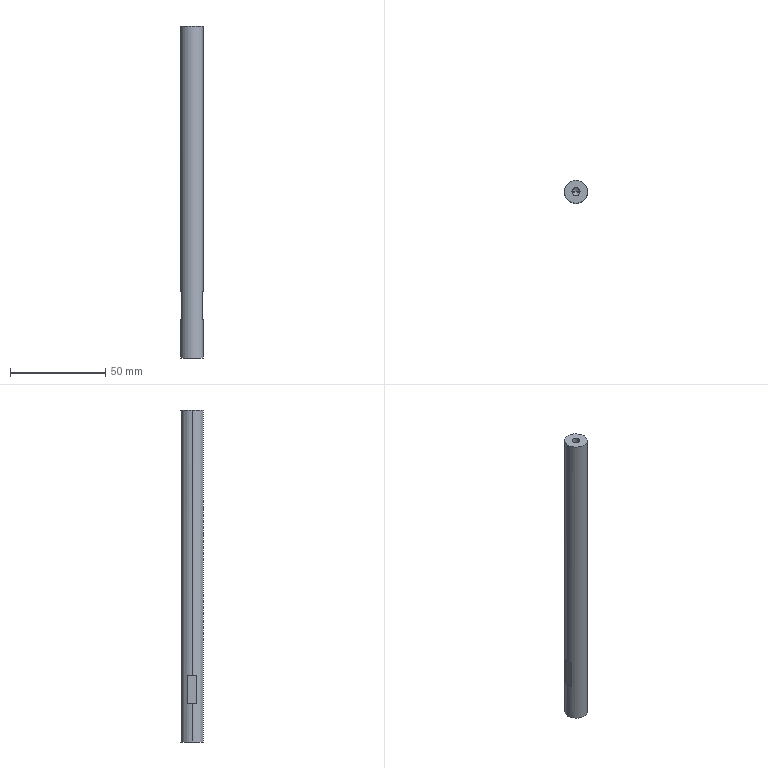Part | STEP file | magnetizing cylinder plate post | 1 solid | 18 faces | box 12 x 12 x 174 mm | volume 19275 mm3 | plane 8 | cylinder 6 | cone 4 | commonest cylinder face diameters 4.2 x4 12 x2
STEP:
#1=CARTESIAN_POINT('',(0.,0.,0.));
#2=DIRECTION('',(0.,0.,1.));
#3=DIRECTION('',(1.,0.,0.));
#4=AXIS2_PLACEMENT_3D('',#1,#2,#3);
#5=CARTESIAN_POINT('',(-2.1,0.,12.4));
#6=VERTEX_POINT('',#5);
#7=CARTESIAN_POINT('',(-2.1,0.,0.));
#8=VERTEX_POINT('',#7);
#9=CARTESIAN_POINT('',(-2.1,0.,0.));
#10=DIRECTION('',(0.,0.,-1.));
#11=VECTOR('',#10,1.);
#12=LINE('',#9,#11);
#13=CARTESIAN_POINT('',(0.,0.,0.));
#14=DIRECTION('',(0.,0.,-1.));
#15=DIRECTION('',(-1.,0.,0.));
#16=AXIS2_PLACEMENT_3D('',#13,#14,#15);
#17=CYLINDRICAL_SURFACE('',#16,2.1);
#18=CARTESIAN_POINT('',(6.283,0.));
#19=DIRECTION('',(0.,1.));
#20=VECTOR('',#19,1.);
#21=LINE('',#18,#20);
#22=(GEOMETRIC_REPRESENTATION_CONTEXT(2)PARAMETRIC_REPRESENTATION_CONTEXT()REPRESENTATION_CONTEXT('',''));
#23=DEFINITIONAL_REPRESENTATION('',(#21),#22);
#24=PCURVE('',#17,#23);
#25=CARTESIAN_POINT('',(0.,0.,0.));
#26=DIRECTION('',(0.,0.,-1.));
#27=DIRECTION('',(-1.,0.,0.));
#28=AXIS2_PLACEMENT_3D('',#25,#26,#27);
#29=CYLINDRICAL_SURFACE('',#28,2.1);
#30=CARTESIAN_POINT('',(0.,0.));
#31=DIRECTION('',(0.,1.));
#32=VECTOR('',#31,1.);
#33=LINE('',#30,#32);
#34=(GEOMETRIC_REPRESENTATION_CONTEXT(2)PARAMETRIC_REPRESENTATION_CONTEXT()REPRESENTATION_CONTEXT('',''));
#35=DEFINITIONAL_REPRESENTATION('',(#33),#34);
#36=PCURVE('',#29,#35);
#37=SURFACE_CURVE('',#12,(#24,#36),.PCURVE_S1.);
#38=EDGE_CURVE('',#6,#8,#37,.T.);
#39=ORIENTED_EDGE('',*,*,#38,.T.);
#40=CARTESIAN_POINT('',(2.1,0.,0.));
#41=VERTEX_POINT('',#40);
#42=CARTESIAN_POINT('',(0.,0.,0.));
#43=DIRECTION('',(0.,0.,-1.));
#44=DIRECTION('',(-1.,0.,0.));
#45=AXIS2_PLACEMENT_3D('',#42,#43,#44);
#46=CIRCLE('',#45,2.1);
#47=CARTESIAN_POINT('',(0.,0.));
#48=DIRECTION('',(1.,0.));
#49=VECTOR('',#48,1.);
#50=LINE('',#47,#49);
#51=(GEOMETRIC_REPRESENTATION_CONTEXT(2)PARAMETRIC_REPRESENTATION_CONTEXT()REPRESENTATION_CONTEXT('',''));
#52=DEFINITIONAL_REPRESENTATION('',(#50),#51);
#53=PCURVE('',#17,#52);
#54=CARTESIAN_POINT('',(0.,0.,0.));
#55=DIRECTION('',(0.,0.,1.));
#56=DIRECTION('',(1.,0.,0.));
#57=AXIS2_PLACEMENT_3D('',#54,#55,#56);
#58=PLANE('',#57);
#59=CARTESIAN_POINT('',(-2.1,0.));
#60=CARTESIAN_POINT('',(-2.1,3.637));
#61=CARTESIAN_POINT('',(1.05,1.819));
#62=CARTESIAN_POINT('',(4.2,0.));
#63=CARTESIAN_POINT('',(1.05,-1.819));
#64=CARTESIAN_POINT('',(-2.1,-3.637));
#65=CARTESIAN_POINT('',(-2.1,0.));
#66=(BOUNDED_CURVE()B_SPLINE_CURVE(2,(#59,#60,#61,#62,#63,#64,#65),.UNSPECIFIED.,.T.,.F.)B_SPLINE_CURVE_WITH_KNOTS((1,2,2,2,2,1),(-2.094,0.,2.094,4.189,6.283,8.378),.UNSPECIFIED.)CURVE()GEOMETRIC_REPRESENTATION_ITEM()RATIONAL_B_SPLINE_CURVE((1.,0.5,1.,0.5,1.,0.5,1.))REPRESENTATION_ITEM(''));
#67=(GEOMETRIC_REPRESENTATION_CONTEXT(2)PARAMETRIC_REPRESENTATION_CONTEXT()REPRESENTATION_CONTEXT('',''));
#68=DEFINITIONAL_REPRESENTATION('',(#66),#67);
#69=PCURVE('',#58,#68);
#70=SURFACE_CURVE('',#46,(#53,#69),.PCURVE_S1.);
#71=EDGE_CURVE('',#41,#8,#70,.T.);
#72=ORIENTED_EDGE('',*,*,#71,.F.);
#73=CARTESIAN_POINT('',(2.1,0.,12.4));
#74=VERTEX_POINT('',#73);
#75=CARTESIAN_POINT('',(2.1,0.,0.));
#76=DIRECTION('',(0.,0.,-1.));
#77=VECTOR('',#76,1.);
#78=LINE('',#75,#77);
#79=CARTESIAN_POINT('',(3.142,0.));
#80=DIRECTION('',(0.,1.));
#81=VECTOR('',#80,1.);
#82=LINE('',#79,#81);
#83=(GEOMETRIC_REPRESENTATION_CONTEXT(2)PARAMETRIC_REPRESENTATION_CONTEXT()REPRESENTATION_CONTEXT('',''));
#84=DEFINITIONAL_REPRESENTATION('',(#82),#83);
#85=PCURVE('',#17,#84);
#86=CARTESIAN_POINT('',(3.142,0.));
#87=DIRECTION('',(0.,1.));
#88=VECTOR('',#87,1.);
#89=LINE('',#86,#88);
#90=(GEOMETRIC_REPRESENTATION_CONTEXT(2)PARAMETRIC_REPRESENTATION_CONTEXT()REPRESENTATION_CONTEXT('',''));
#91=DEFINITIONAL_REPRESENTATION('',(#89),#90);
#92=PCURVE('',#29,#91);
#93=SURFACE_CURVE('',#78,(#85,#92),.PCURVE_S1.);
#94=EDGE_CURVE('',#74,#41,#93,.T.);
#95=ORIENTED_EDGE('',*,*,#94,.F.);
#96=CARTESIAN_POINT('',(0.,0.,12.4));
#97=DIRECTION('',(0.,0.,-1.));
#98=DIRECTION('',(-1.,0.,0.));
#99=AXIS2_PLACEMENT_3D('',#96,#97,#98);
#100=CIRCLE('',#99,2.1);
#101=CARTESIAN_POINT('',(0.,-12.4));
#102=DIRECTION('',(1.,0.));
#103=VECTOR('',#102,1.);
#104=LINE('',#101,#103);
#105=(GEOMETRIC_REPRESENTATION_CONTEXT(2)PARAMETRIC_REPRESENTATION_CONTEXT()REPRESENTATION_CONTEXT('',''));
#106=DEFINITIONAL_REPRESENTATION('',(#104),#105);
#107=PCURVE('',#17,#106);
#108=CARTESIAN_POINT('',(0.,0.,12.4));
#109=DIRECTION('',(0.,0.,-1.));
#110=DIRECTION('',(-1.,0.,0.));
#111=AXIS2_PLACEMENT_3D('',#108,#109,#110);
#112=CONICAL_SURFACE('',#111,2.1,1.03);
#113=CARTESIAN_POINT('',(0.,0.));
#114=DIRECTION('',(1.,0.));
#115=VECTOR('',#114,1.);
#116=LINE('',#113,#115);
#117=(GEOMETRIC_REPRESENTATION_CONTEXT(2)PARAMETRIC_REPRESENTATION_CONTEXT()REPRESENTATION_CONTEXT('',''));
#118=DEFINITIONAL_REPRESENTATION('',(#116),#117);
#119=PCURVE('',#112,#118);
#120=SURFACE_CURVE('',#100,(#107,#119),.PCURVE_S1.);
#121=EDGE_CURVE('',#74,#6,#120,.T.);
#122=ORIENTED_EDGE('',*,*,#121,.T.);
#123=EDGE_LOOP('',(#39,#72,#95,#122));
#124=FACE_BOUND('',#123,.F.);
#125=ADVANCED_FACE('',(#124),#17,.F.);
#126=ORIENTED_EDGE('',*,*,#121,.F.);
#127=CARTESIAN_POINT('',(0.,0.,13.662));
#128=VERTEX_POINT('',#127);
#129=CARTESIAN_POINT('',(2.1,0.,12.4));
#130=DIRECTION('',(0.8572,0.,-0.515));
#131=VECTOR('',#130,1.);
#132=LINE('',#129,#131);
#133=CARTESIAN_POINT('',(3.142,0.));
#134=DIRECTION('',(0.,1.));
#135=VECTOR('',#134,1.);
#136=LINE('',#133,#135);
#137=(GEOMETRIC_REPRESENTATION_CONTEXT(2)PARAMETRIC_REPRESENTATION_CONTEXT()REPRESENTATION_CONTEXT('',''));
#138=DEFINITIONAL_REPRESENTATION('',(#136),#137);
#139=PCURVE('',#112,#138);
#140=CARTESIAN_POINT('',(0.,0.,12.4));
#141=DIRECTION('',(0.,0.,-1.));
#142=DIRECTION('',(-1.,0.,0.));
#143=AXIS2_PLACEMENT_3D('',#140,#141,#142);
#144=CONICAL_SURFACE('',#143,2.1,1.03);
#145=CARTESIAN_POINT('',(3.142,0.));
#146=DIRECTION('',(0.,1.));
#147=VECTOR('',#146,1.);
#148=LINE('',#145,#147);
#149=(GEOMETRIC_REPRESENTATION_CONTEXT(2)PARAMETRIC_REPRESENTATION_CONTEXT()REPRESENTATION_CONTEXT('',''));
#150=DEFINITIONAL_REPRESENTATION('',(#148),#149);
#151=PCURVE('',#144,#150);
#152=SURFACE_CURVE('',#132,(#139,#151),.PCURVE_S1.);
#153=EDGE_CURVE('',#128,#74,#152,.T.);
#154=ORIENTED_EDGE('',*,*,#153,.F.);
#155=CARTESIAN_POINT('',(-2.1,0.,12.4));
#156=DIRECTION('',(-0.8572,0.,-0.515));
#157=VECTOR('',#156,1.);
#158=LINE('',#155,#157);
#159=CARTESIAN_POINT('',(6.283,0.));
#160=DIRECTION('',(0.,1.));
#161=VECTOR('',#160,1.);
#162=LINE('',#159,#161);
#163=(GEOMETRIC_REPRESENTATION_CONTEXT(2)PARAMETRIC_REPRESENTATION_CONTEXT()REPRESENTATION_CONTEXT('',''));
#164=DEFINITIONAL_REPRESENTATION('',(#162),#163);
#165=PCURVE('',#112,#164);
#166=CARTESIAN_POINT('',(0.,0.));
#167=DIRECTION('',(0.,1.));
#168=VECTOR('',#167,1.);
#169=LINE('',#166,#168);
#170=(GEOMETRIC_REPRESENTATION_CONTEXT(2)PARAMETRIC_REPRESENTATION_CONTEXT()REPRESENTATION_CONTEXT('',''));
#171=DEFINITIONAL_REPRESENTATION('',(#169),#170);
#172=PCURVE('',#144,#171);
#173=SURFACE_CURVE('',#158,(#165,#172),.PCURVE_S1.);
#174=EDGE_CURVE('',#128,#6,#173,.T.);
#175=ORIENTED_EDGE('',*,*,#174,.T.);
#176=EDGE_LOOP('',(#126,#154,#175));
#177=FACE_BOUND('',#176,.F.);
#178=ADVANCED_FACE('',(#177),#112,.F.);
#179=CARTESIAN_POINT('',(2.1,0.,161.6));
#180=VERTEX_POINT('',#179);
#181=CARTESIAN_POINT('',(2.1,0.,174.));
#182=VERTEX_POINT('',#181);
#183=CARTESIAN_POINT('',(2.1,0.,174.));
#184=DIRECTION('',(0.,0.,1.));
#185=VECTOR('',#184,1.);
#186=LINE('',#183,#185);
#187=CARTESIAN_POINT('',(0.,0.,174.));
#188=DIRECTION('',(0.,0.,1.));
#189=DIRECTION('',(1.,0.,0.));
#190=AXIS2_PLACEMENT_3D('',#187,#188,#189);
#191=CYLINDRICAL_SURFACE('',#190,2.1);
#192=CARTESIAN_POINT('',(6.283,0.));
#193=DIRECTION('',(0.,1.));
#194=VECTOR('',#193,1.);
#195=LINE('',#192,#194);
#196=(GEOMETRIC_REPRESENTATION_CONTEXT(2)PARAMETRIC_REPRESENTATION_CONTEXT()REPRESENTATION_CONTEXT('',''));
#197=DEFINITIONAL_REPRESENTATION('',(#195),#196);
#198=PCURVE('',#191,#197);
#199=CARTESIAN_POINT('',(0.,0.,174.));
#200=DIRECTION('',(0.,0.,1.));
#201=DIRECTION('',(1.,0.,0.));
#202=AXIS2_PLACEMENT_3D('',#199,#200,#201);
#203=CYLINDRICAL_SURFACE('',#202,2.1);
#204=CARTESIAN_POINT('',(0.,0.));
#205=DIRECTION('',(0.,1.));
#206=VECTOR('',#205,1.);
#207=LINE('',#204,#206);
#208=(GEOMETRIC_REPRESENTATION_CONTEXT(2)PARAMETRIC_REPRESENTATION_CONTEXT()REPRESENTATION_CONTEXT('',''));
#209=DEFINITIONAL_REPRESENTATION('',(#207),#208);
#210=PCURVE('',#203,#209);
#211=SURFACE_CURVE('',#186,(#198,#210),.PCURVE_S1.);
#212=EDGE_CURVE('',#180,#182,#211,.T.);
#213=ORIENTED_EDGE('',*,*,#212,.T.);
#214=CARTESIAN_POINT('',(-2.1,0.,174.));
#215=VERTEX_POINT('',#214);
#216=CARTESIAN_POINT('',(0.,0.,174.));
#217=DIRECTION('',(0.,0.,1.));
#218=DIRECTION('',(1.,0.,0.));
#219=AXIS2_PLACEMENT_3D('',#216,#217,#218);
#220=CIRCLE('',#219,2.1);
#221=CARTESIAN_POINT('',(0.,0.));
#222=DIRECTION('',(1.,0.));
#223=VECTOR('',#222,1.);
#224=LINE('',#221,#223);
#225=(GEOMETRIC_REPRESENTATION_CONTEXT(2)PARAMETRIC_REPRESENTATION_CONTEXT()REPRESENTATION_CONTEXT('',''));
#226=DEFINITIONAL_REPRESENTATION('',(#224),#225);
#227=PCURVE('',#191,#226);
#228=CARTESIAN_POINT('',(0.,0.,174.));
#229=DIRECTION('',(0.,0.,1.));
#230=DIRECTION('',(1.,0.,0.));
#231=AXIS2_PLACEMENT_3D('',#228,#229,#230);
#232=PLANE('',#231);
#233=CARTESIAN_POINT('',(0.,0.));
#234=DIRECTION('',(1.,0.));
#235=AXIS2_PLACEMENT_2D('',#233,#234);
#236=CIRCLE('',#235,2.1);
#237=(GEOMETRIC_REPRESENTATION_CONTEXT(2)PARAMETRIC_REPRESENTATION_CONTEXT()REPRESENTATION_CONTEXT('',''));
#238=DEFINITIONAL_REPRESENTATION('',(#236),#237);
#239=PCURVE('',#232,#238);
#240=SURFACE_CURVE('',#220,(#227,#239),.PCURVE_S1.);
#241=EDGE_CURVE('',#215,#182,#240,.T.);
#242=ORIENTED_EDGE('',*,*,#241,.F.);
#243=CARTESIAN_POINT('',(-2.1,0.,161.6));
#244=VERTEX_POINT('',#243);
#245=CARTESIAN_POINT('',(-2.1,0.,174.));
#246=DIRECTION('',(0.,0.,1.));
#247=VECTOR('',#246,1.);
#248=LINE('',#245,#247);
#249=CARTESIAN_POINT('',(3.142,0.));
#250=DIRECTION('',(0.,1.));
#251=VECTOR('',#250,1.);
#252=LINE('',#249,#251);
#253=(GEOMETRIC_REPRESENTATION_CONTEXT(2)PARAMETRIC_REPRESENTATION_CONTEXT()REPRESENTATION_CONTEXT('',''));
#254=DEFINITIONAL_REPRESENTATION('',(#252),#253);
#255=PCURVE('',#191,#254);
#256=CARTESIAN_POINT('',(3.142,0.));
#257=DIRECTION('',(0.,1.));
#258=VECTOR('',#257,1.);
#259=LINE('',#256,#258);
#260=(GEOMETRIC_REPRESENTATION_CONTEXT(2)PARAMETRIC_REPRESENTATION_CONTEXT()REPRESENTATION_CONTEXT('',''));
#261=DEFINITIONAL_REPRESENTATION('',(#259),#260);
#262=PCURVE('',#203,#261);
#263=SURFACE_CURVE('',#248,(#255,#262),.PCURVE_S1.);
#264=EDGE_CURVE('',#244,#215,#263,.T.);
#265=ORIENTED_EDGE('',*,*,#264,.F.);
#266=CARTESIAN_POINT('',(0.,0.,161.6));
#267=DIRECTION('',(0.,0.,1.));
#268=DIRECTION('',(1.,0.,0.));
#269=AXIS2_PLACEMENT_3D('',#266,#267,#268);
#270=CIRCLE('',#269,2.1);
#271=CARTESIAN_POINT('',(0.,-12.4));
#272=DIRECTION('',(1.,0.));
#273=VECTOR('',#272,1.);
#274=LINE('',#271,#273);
#275=(GEOMETRIC_REPRESENTATION_CONTEXT(2)PARAMETRIC_REPRESENTATION_CONTEXT()REPRESENTATION_CONTEXT('',''));
#276=DEFINITIONAL_REPRESENTATION('',(#274),#275);
#277=PCURVE('',#191,#276);
#278=CARTESIAN_POINT('',(0.,0.,161.6));
#279=DIRECTION('',(0.,0.,1.));
#280=DIRECTION('',(1.,0.,0.));
#281=AXIS2_PLACEMENT_3D('',#278,#279,#280);
#282=CONICAL_SURFACE('',#281,2.1,1.03);
#283=CARTESIAN_POINT('',(0.,0.));
#284=DIRECTION('',(1.,0.));
#285=VECTOR('',#284,1.);
#286=LINE('',#283,#285);
#287=(GEOMETRIC_REPRESENTATION_CONTEXT(2)PARAMETRIC_REPRESENTATION_CONTEXT()REPRESENTATION_CONTEXT('',''));
#288=DEFINITIONAL_REPRESENTATION('',(#286),#287);
#289=PCURVE('',#282,#288);
#290=SURFACE_CURVE('',#270,(#277,#289),.PCURVE_S1.);
#291=EDGE_CURVE('',#244,#180,#290,.T.);
#292=ORIENTED_EDGE('',*,*,#291,.T.);
#293=EDGE_LOOP('',(#213,#242,#265,#292));
#294=FACE_BOUND('',#293,.F.);
#295=ADVANCED_FACE('',(#294),#191,.F.);
#296=ORIENTED_EDGE('',*,*,#291,.F.);
#297=CARTESIAN_POINT('',(0.,0.,160.338));
#298=VERTEX_POINT('',#297);
#299=CARTESIAN_POINT('',(-2.1,0.,161.6));
#300=DIRECTION('',(-0.8572,0.,0.515));
#301=VECTOR('',#300,1.);
#302=LINE('',#299,#301);
#303=CARTESIAN_POINT('',(3.142,0.));
#304=DIRECTION('',(0.,1.));
#305=VECTOR('',#304,1.);
#306=LINE('',#303,#305);
#307=(GEOMETRIC_REPRESENTATION_CONTEXT(2)PARAMETRIC_REPRESENTATION_CONTEXT()REPRESENTATION_CONTEXT('',''));
#308=DEFINITIONAL_REPRESENTATION('',(#306),#307);
#309=PCURVE('',#282,#308);
#310=CARTESIAN_POINT('',(0.,0.,161.6));
#311=DIRECTION('',(0.,0.,1.));
#312=DIRECTION('',(1.,0.,0.));
#313=AXIS2_PLACEMENT_3D('',#310,#311,#312);
#314=CONICAL_SURFACE('',#313,2.1,1.03);
#315=CARTESIAN_POINT('',(3.142,0.));
#316=DIRECTION('',(0.,1.));
#317=VECTOR('',#316,1.);
#318=LINE('',#315,#317);
#319=(GEOMETRIC_REPRESENTATION_CONTEXT(2)PARAMETRIC_REPRESENTATION_CONTEXT()REPRESENTATION_CONTEXT('',''));
#320=DEFINITIONAL_REPRESENTATION('',(#318),#319);
#321=PCURVE('',#314,#320);
#322=SURFACE_CURVE('',#302,(#309,#321),.PCURVE_S1.);
#323=EDGE_CURVE('',#298,#244,#322,.T.);
#324=ORIENTED_EDGE('',*,*,#323,.F.);
#325=CARTESIAN_POINT('',(2.1,0.,161.6));
#326=DIRECTION('',(0.8572,0.,0.515));
#327=VECTOR('',#326,1.);
#328=LINE('',#325,#327);
#329=CARTESIAN_POINT('',(6.283,-1.262));
#330=CARTESIAN_POINT('',(6.283,-1.243));
#331=CARTESIAN_POINT('',(6.283,-1.204));
#332=CARTESIAN_POINT('',(6.283,-1.147));
#333=CARTESIAN_POINT('',(6.283,-1.09));
#334=CARTESIAN_POINT('',(6.283,-1.032));
#335=CARTESIAN_POINT('',(6.283,-0.975));
#336=CARTESIAN_POINT('',(6.283,-0.9177));
#337=CARTESIAN_POINT('',(6.283,-0.8603));
#338=CARTESIAN_POINT('',(6.283,-0.803));
#339=CARTESIAN_POINT('',(6.283,-0.7456));
#340=CARTESIAN_POINT('',(6.283,-0.6883));
#341=CARTESIAN_POINT('',(6.283,-0.6309));
#342=CARTESIAN_POINT('',(6.283,-0.5735));
#343=CARTESIAN_POINT('',(6.283,-0.5162));
#344=CARTESIAN_POINT('',(6.283,-0.4588));
#345=CARTESIAN_POINT('',(6.283,-0.4015));
#346=CARTESIAN_POINT('',(6.283,-0.3441));
#347=CARTESIAN_POINT('',(6.283,-0.2868));
#348=CARTESIAN_POINT('',(6.283,-0.2294));
#349=CARTESIAN_POINT('',(6.283,-0.1721));
#350=CARTESIAN_POINT('',(6.283,-0.1147));
#351=CARTESIAN_POINT('',(6.283,-0.05735));
#352=CARTESIAN_POINT('',(6.283,-0.01912));
#353=CARTESIAN_POINT('',(6.283,0.));
#354=B_SPLINE_CURVE_WITH_KNOTS('',3,(#329,#330,#331,#332,#333,#334,#335,#336,#337,#338,#339,#340,#341,#342,#343,#344,#345,#346,#347,#348,#349,#350,#351,#352,#353),.UNSPECIFIED.,.F.,.F.,(4,1,1,1,1,1,1,1,1,1,1,1,1,1,1,1,1,1,1,1,1,1,4),(-2.45,-2.339,-2.227,-2.116,-2.004,-1.893,-1.782,-1.67,-1.559,-1.448,-1.336,-1.225,-1.114,-1.002,-0.8909,-0.7795,-0.6682,-0.5568,-0.4454,-0.3341,-0.2227,-0.1114,0.),.UNSPECIFIED.);
#355=(GEOMETRIC_REPRESENTATION_CONTEXT(2)PARAMETRIC_REPRESENTATION_CONTEXT()REPRESENTATION_CONTEXT('',''));
#356=DEFINITIONAL_REPRESENTATION('',(#354),#355);
#357=PCURVE('',#282,#356);
#358=CARTESIAN_POINT('',(0.,-1.262));
#359=CARTESIAN_POINT('',(0.,-1.243));
#360=CARTESIAN_POINT('',(0.,-1.204));
#361=CARTESIAN_POINT('',(0.,-1.147));
#362=CARTESIAN_POINT('',(0.,-1.09));
#363=CARTESIAN_POINT('',(0.,-1.032));
#364=CARTESIAN_POINT('',(0.,-0.975));
#365=CARTESIAN_POINT('',(0.,-0.9177));
#366=CARTESIAN_POINT('',(0.,-0.8603));
#367=CARTESIAN_POINT('',(0.,-0.803));
#368=CARTESIAN_POINT('',(0.,-0.7456));
#369=CARTESIAN_POINT('',(0.,-0.6883));
#370=CARTESIAN_POINT('',(0.,-0.6309));
#371=CARTESIAN_POINT('',(0.,-0.5735));
#372=CARTESIAN_POINT('',(0.,-0.5162));
#373=CARTESIAN_POINT('',(0.,-0.4588));
#374=CARTESIAN_POINT('',(0.,-0.4015));
#375=CARTESIAN_POINT('',(0.,-0.3441));
#376=CARTESIAN_POINT('',(0.,-0.2868));
#377=CARTESIAN_POINT('',(0.,-0.2294));
#378=CARTESIAN_POINT('',(0.,-0.1721));
#379=CARTESIAN_POINT('',(0.,-0.1147));
#380=CARTESIAN_POINT('',(0.,-0.05735));
#381=CARTESIAN_POINT('',(0.,-0.01912));
#382=CARTESIAN_POINT('',(0.,0.));
#383=B_SPLINE_CURVE_WITH_KNOTS('',3,(#358,#359,#360,#361,#362,#363,#364,#365,#366,#367,#368,#369,#370,#371,#372,#373,#374,#375,#376,#377,#378,#379,#380,#381,#382),.UNSPECIFIED.,.F.,.F.,(4,1,1,1,1,1,1,1,1,1,1,1,1,1,1,1,1,1,1,1,1,1,4),(-2.45,-2.339,-2.227,-2.116,-2.004,-1.893,-1.782,-1.67,-1.559,-1.448,-1.336,-1.225,-1.114,-1.002,-0.8909,-0.7795,-0.6682,-0.5568,-0.4454,-0.3341,-0.2227,-0.1114,0.),.UNSPECIFIED.);
#384=(GEOMETRIC_REPRESENTATION_CONTEXT(2)PARAMETRIC_REPRESENTATION_CONTEXT()REPRESENTATION_CONTEXT('',''));
#385=DEFINITIONAL_REPRESENTATION('',(#383),#384);
#386=PCURVE('',#314,#385);
#387=SURFACE_CURVE('',#328,(#357,#386),.PCURVE_S1.);
#388=EDGE_CURVE('',#298,#180,#387,.T.);
#389=ORIENTED_EDGE('',*,*,#388,.T.);
#390=EDGE_LOOP('',(#296,#324,#389));
#391=FACE_BOUND('',#390,.F.);
#392=ADVANCED_FACE('',(#391),#282,.F.);
#393=CARTESIAN_POINT('',(6.,0.,174.));
#394=VERTEX_POINT('',#393);
#395=CARTESIAN_POINT('',(-6.,0.,174.));
#396=VERTEX_POINT('',#395);
#397=CARTESIAN_POINT('',(0.,0.,174.));
#398=DIRECTION('',(0.,0.,1.));
#399=DIRECTION('',(1.,0.,0.));
#400=AXIS2_PLACEMENT_3D('',#397,#398,#399);
#401=CIRCLE('',#400,6.);
#402=CARTESIAN_POINT('',(0.,0.,174.));
#403=DIRECTION('',(0.,0.,-1.));
#404=DIRECTION('',(-1.,0.,0.));
#405=AXIS2_PLACEMENT_3D('',#402,#403,#404);
#406=CYLINDRICAL_SURFACE('',#405,6.);
#407=CARTESIAN_POINT('',(3.142,0.));
#408=DIRECTION('',(-1.,0.));
#409=VECTOR('',#408,1.);
#410=LINE('',#407,#409);
#411=(GEOMETRIC_REPRESENTATION_CONTEXT(2)PARAMETRIC_REPRESENTATION_CONTEXT()REPRESENTATION_CONTEXT('',''));
#412=DEFINITIONAL_REPRESENTATION('',(#410),#411);
#413=PCURVE('',#406,#412);
#414=CARTESIAN_POINT('',(0.,0.));
#415=DIRECTION('',(1.,0.));
#416=AXIS2_PLACEMENT_2D('',#414,#415);
#417=CIRCLE('',#416,6.);
#418=(GEOMETRIC_REPRESENTATION_CONTEXT(2)PARAMETRIC_REPRESENTATION_CONTEXT()REPRESENTATION_CONTEXT('',''));
#419=DEFINITIONAL_REPRESENTATION('',(#417),#418);
#420=PCURVE('',#232,#419);
#421=SURFACE_CURVE('',#401,(#413,#420),.PCURVE_S1.);
#422=EDGE_CURVE('',#394,#396,#421,.T.);
#423=ORIENTED_EDGE('',*,*,#422,.F.);
#424=CARTESIAN_POINT('',(6.,0.,35.));
#425=VERTEX_POINT('',#424);
#426=CARTESIAN_POINT('',(6.,0.,174.));
#427=DIRECTION('',(0.,0.,-1.));
#428=VECTOR('',#427,1.);
#429=LINE('',#426,#428);
#430=CARTESIAN_POINT('',(3.142,0.));
#431=DIRECTION('',(0.,1.));
#432=VECTOR('',#431,1.);
#433=LINE('',#430,#432);
#434=(GEOMETRIC_REPRESENTATION_CONTEXT(2)PARAMETRIC_REPRESENTATION_CONTEXT()REPRESENTATION_CONTEXT('',''));
#435=DEFINITIONAL_REPRESENTATION('',(#433),#434);
#436=PCURVE('',#406,#435);
#437=CARTESIAN_POINT('',(0.,0.,174.));
#438=DIRECTION('',(0.,0.,-1.));
#439=DIRECTION('',(-1.,0.,0.));
#440=AXIS2_PLACEMENT_3D('',#437,#438,#439);
#441=CYLINDRICAL_SURFACE('',#440,6.);
#442=CARTESIAN_POINT('',(3.142,0.));
#443=DIRECTION('',(0.,1.));
#444=VECTOR('',#443,1.);
#445=LINE('',#442,#444);
#446=(GEOMETRIC_REPRESENTATION_CONTEXT(2)PARAMETRIC_REPRESENTATION_CONTEXT()REPRESENTATION_CONTEXT('',''));
#447=DEFINITIONAL_REPRESENTATION('',(#445),#446);
#448=PCURVE('',#441,#447);
#449=SURFACE_CURVE('',#429,(#436,#448),.PCURVE_S1.);
#450=EDGE_CURVE('',#394,#425,#449,.T.);
#451=ORIENTED_EDGE('',*,*,#450,.T.);
#452=CARTESIAN_POINT('',(5.5,2.398,35.));
#453=VERTEX_POINT('',#452);
#454=CARTESIAN_POINT('',(0.,0.,35.));
#455=DIRECTION('',(0.,0.,-1.));
#456=DIRECTION('',(-1.,0.,0.));
#457=AXIS2_PLACEMENT_3D('',#454,#455,#456);
#458=CIRCLE('',#457,6.);
#459=CARTESIAN_POINT('',(0.,139.));
#460=DIRECTION('',(1.,0.));
#461=VECTOR('',#460,1.);
#462=LINE('',#459,#461);
#463=(GEOMETRIC_REPRESENTATION_CONTEXT(2)PARAMETRIC_REPRESENTATION_CONTEXT()REPRESENTATION_CONTEXT('',''));
#464=DEFINITIONAL_REPRESENTATION('',(#462),#463);
#465=PCURVE('',#406,#464);
#466=CARTESIAN_POINT('',(5.5,186.,35.));
#467=DIRECTION('',(0.,0.,-1.));
#468=DIRECTION('',(-1.,0.,0.));
#469=AXIS2_PLACEMENT_3D('',#466,#467,#468);
#470=PLANE('',#469);
#471=CARTESIAN_POINT('',(5.5,-186.));
#472=DIRECTION('',(1.,0.));
#473=AXIS2_PLACEMENT_2D('',#471,#472);
#474=CIRCLE('',#473,6.);
#475=(GEOMETRIC_REPRESENTATION_CONTEXT(2)PARAMETRIC_REPRESENTATION_CONTEXT()REPRESENTATION_CONTEXT('',''));
#476=DEFINITIONAL_REPRESENTATION('',(#474),#475);
#477=PCURVE('',#470,#476);
#478=SURFACE_CURVE('',#458,(#465,#477),.PCURVE_S1.);
#479=EDGE_CURVE('',#453,#425,#478,.T.);
#480=ORIENTED_EDGE('',*,*,#479,.F.);
#481=CARTESIAN_POINT('',(5.5,2.398,20.));
#482=VERTEX_POINT('',#481);
#483=CARTESIAN_POINT('',(5.5,2.398,174.));
#484=DIRECTION('',(0.,0.,1.));
#485=VECTOR('',#484,1.);
#486=LINE('',#483,#485);
#487=CARTESIAN_POINT('',(2.73,0.));
#488=DIRECTION('',(0.,-1.));
#489=VECTOR('',#488,1.);
#490=LINE('',#487,#489);
#491=(GEOMETRIC_REPRESENTATION_CONTEXT(2)PARAMETRIC_REPRESENTATION_CONTEXT()REPRESENTATION_CONTEXT('',''));
#492=DEFINITIONAL_REPRESENTATION('',(#490),#491);
#493=PCURVE('',#406,#492);
#494=CARTESIAN_POINT('',(5.5,186.,20.));
#495=DIRECTION('',(1.,0.,0.));
#496=DIRECTION('',(0.,0.,-1.));
#497=AXIS2_PLACEMENT_3D('',#494,#495,#496);
#498=PLANE('',#497);
#499=CARTESIAN_POINT('',(-154.,-183.602));
#500=DIRECTION('',(-1.,0.));
#501=VECTOR('',#500,1.);
#502=LINE('',#499,#501);
#503=(GEOMETRIC_REPRESENTATION_CONTEXT(2)PARAMETRIC_REPRESENTATION_CONTEXT()REPRESENTATION_CONTEXT('',''));
#504=DEFINITIONAL_REPRESENTATION('',(#502),#503);
#505=PCURVE('',#498,#504);
#506=SURFACE_CURVE('',#486,(#493,#505),.PCURVE_S1.);
#507=EDGE_CURVE('',#482,#453,#506,.T.);
#508=ORIENTED_EDGE('',*,*,#507,.F.);
#509=CARTESIAN_POINT('',(6.,0.,20.));
#510=VERTEX_POINT('',#509);
#511=CARTESIAN_POINT('',(0.,0.,20.));
#512=DIRECTION('',(0.,0.,1.));
#513=DIRECTION('',(1.,0.,0.));
#514=AXIS2_PLACEMENT_3D('',#511,#512,#513);
#515=CIRCLE('',#514,6.);
#516=CARTESIAN_POINT('',(3.142,154.));
#517=DIRECTION('',(-1.,0.));
#518=VECTOR('',#517,1.);
#519=LINE('',#516,#518);
#520=(GEOMETRIC_REPRESENTATION_CONTEXT(2)PARAMETRIC_REPRESENTATION_CONTEXT()REPRESENTATION_CONTEXT('',''));
#521=DEFINITIONAL_REPRESENTATION('',(#519),#520);
#522=PCURVE('',#406,#521);
#523=CARTESIAN_POINT('',(5.5,186.,20.));
#524=DIRECTION('',(0.,0.,1.));
#525=DIRECTION('',(1.,0.,0.));
#526=AXIS2_PLACEMENT_3D('',#523,#524,#525);
#527=PLANE('',#526);
#528=CARTESIAN_POINT('',(-5.5,-186.));
#529=DIRECTION('',(1.,0.));
#530=AXIS2_PLACEMENT_2D('',#528,#529);
#531=CIRCLE('',#530,6.);
#532=(GEOMETRIC_REPRESENTATION_CONTEXT(2)PARAMETRIC_REPRESENTATION_CONTEXT()REPRESENTATION_CONTEXT('',''));
#533=DEFINITIONAL_REPRESENTATION('',(#531),#532);
#534=PCURVE('',#527,#533);
#535=SURFACE_CURVE('',#515,(#522,#534),.PCURVE_S1.);
#536=EDGE_CURVE('',#510,#482,#535,.T.);
#537=ORIENTED_EDGE('',*,*,#536,.F.);
#538=CARTESIAN_POINT('',(6.,0.,0.));
#539=VERTEX_POINT('',#538);
#540=CARTESIAN_POINT('',(6.,0.,174.));
#541=DIRECTION('',(0.,0.,-1.));
#542=VECTOR('',#541,1.);
#543=LINE('',#540,#542);
#544=CARTESIAN_POINT('',(3.142,0.));
#545=DIRECTION('',(0.,1.));
#546=VECTOR('',#545,1.);
#547=LINE('',#544,#546);
#548=(GEOMETRIC_REPRESENTATION_CONTEXT(2)PARAMETRIC_REPRESENTATION_CONTEXT()REPRESENTATION_CONTEXT('',''));
#549=DEFINITIONAL_REPRESENTATION('',(#547),#548);
#550=PCURVE('',#406,#549);
#551=CARTESIAN_POINT('',(3.142,0.));
#552=DIRECTION('',(0.,1.));
#553=VECTOR('',#552,1.);
#554=LINE('',#551,#553);
#555=(GEOMETRIC_REPRESENTATION_CONTEXT(2)PARAMETRIC_REPRESENTATION_CONTEXT()REPRESENTATION_CONTEXT('',''));
#556=DEFINITIONAL_REPRESENTATION('',(#554),#555);
#557=PCURVE('',#441,#556);
#558=SURFACE_CURVE('',#543,(#550,#557),.PCURVE_S1.);
#559=EDGE_CURVE('',#510,#539,#558,.T.);
#560=ORIENTED_EDGE('',*,*,#559,.T.);
#561=CARTESIAN_POINT('',(-6.,0.,0.));
#562=VERTEX_POINT('',#561);
#563=CARTESIAN_POINT('',(0.,0.,0.));
#564=DIRECTION('',(0.,0.,1.));
#565=DIRECTION('',(1.,0.,0.));
#566=AXIS2_PLACEMENT_3D('',#563,#564,#565);
#567=CIRCLE('',#566,6.);
#568=CARTESIAN_POINT('',(3.142,174.));
#569=DIRECTION('',(-1.,0.));
#570=VECTOR('',#569,1.);
#571=LINE('',#568,#570);
#572=(GEOMETRIC_REPRESENTATION_CONTEXT(2)PARAMETRIC_REPRESENTATION_CONTEXT()REPRESENTATION_CONTEXT('',''));
#573=DEFINITIONAL_REPRESENTATION('',(#571),#572);
#574=PCURVE('',#406,#573);
#575=CARTESIAN_POINT('',(0.,0.));
#576=DIRECTION('',(1.,0.));
#577=AXIS2_PLACEMENT_2D('',#575,#576);
#578=CIRCLE('',#577,6.);
#579=(GEOMETRIC_REPRESENTATION_CONTEXT(2)PARAMETRIC_REPRESENTATION_CONTEXT()REPRESENTATION_CONTEXT('',''));
#580=DEFINITIONAL_REPRESENTATION('',(#578),#579);
#581=PCURVE('',#58,#580);
#582=SURFACE_CURVE('',#567,(#574,#581),.PCURVE_S1.);
#583=EDGE_CURVE('',#539,#562,#582,.T.);
#584=ORIENTED_EDGE('',*,*,#583,.T.);
#585=CARTESIAN_POINT('',(-6.,0.,20.));
#586=VERTEX_POINT('',#585);
#587=CARTESIAN_POINT('',(-6.,0.,174.));
#588=DIRECTION('',(0.,0.,-1.));
#589=VECTOR('',#588,1.);
#590=LINE('',#587,#589);
#591=CARTESIAN_POINT('',(0.,0.));
#592=DIRECTION('',(0.,1.));
#593=VECTOR('',#592,1.);
#594=LINE('',#591,#593);
#595=(GEOMETRIC_REPRESENTATION_CONTEXT(2)PARAMETRIC_REPRESENTATION_CONTEXT()REPRESENTATION_CONTEXT('',''));
#596=DEFINITIONAL_REPRESENTATION('',(#594),#595);
#597=PCURVE('',#406,#596);
#598=CARTESIAN_POINT('',(6.283,0.));
#599=DIRECTION('',(0.,1.));
#600=VECTOR('',#599,1.);
#601=LINE('',#598,#600);
#602=(GEOMETRIC_REPRESENTATION_CONTEXT(2)PARAMETRIC_REPRESENTATION_CONTEXT()REPRESENTATION_CONTEXT('',''));
#603=DEFINITIONAL_REPRESENTATION('',(#601),#602);
#604=PCURVE('',#441,#603);
#605=SURFACE_CURVE('',#590,(#597,#604),.PCURVE_S1.);
#606=EDGE_CURVE('',#586,#562,#605,.T.);
#607=ORIENTED_EDGE('',*,*,#606,.F.);
#608=CARTESIAN_POINT('',(-5.5,2.398,20.));
#609=VERTEX_POINT('',#608);
#610=CARTESIAN_POINT('',(0.,0.,20.));
#611=DIRECTION('',(0.,0.,1.));
#612=DIRECTION('',(1.,0.,0.));
#613=AXIS2_PLACEMENT_3D('',#610,#611,#612);
#614=CIRCLE('',#613,6.);
#615=CARTESIAN_POINT('',(3.142,154.));
#616=DIRECTION('',(-1.,0.));
#617=VECTOR('',#616,1.);
#618=LINE('',#615,#617);
#619=(GEOMETRIC_REPRESENTATION_CONTEXT(2)PARAMETRIC_REPRESENTATION_CONTEXT()REPRESENTATION_CONTEXT('',''));
#620=DEFINITIONAL_REPRESENTATION('',(#618),#619);
#621=PCURVE('',#406,#620);
#622=CARTESIAN_POINT('',(-11.935,186.,20.));
#623=DIRECTION('',(0.,0.,1.));
#624=DIRECTION('',(1.,0.,0.));
#625=AXIS2_PLACEMENT_3D('',#622,#623,#624);
#626=PLANE('',#625);
#627=CARTESIAN_POINT('',(11.935,-186.));
#628=DIRECTION('',(1.,0.));
#629=AXIS2_PLACEMENT_2D('',#627,#628);
#630=CIRCLE('',#629,6.);
#631=(GEOMETRIC_REPRESENTATION_CONTEXT(2)PARAMETRIC_REPRESENTATION_CONTEXT()REPRESENTATION_CONTEXT('',''));
#632=DEFINITIONAL_REPRESENTATION('',(#630),#631);
#633=PCURVE('',#626,#632);
#634=SURFACE_CURVE('',#614,(#621,#633),.PCURVE_S1.);
#635=EDGE_CURVE('',#609,#586,#634,.T.);
#636=ORIENTED_EDGE('',*,*,#635,.F.);
#637=CARTESIAN_POINT('',(-5.5,2.398,35.));
#638=VERTEX_POINT('',#637);
#639=CARTESIAN_POINT('',(-5.5,2.398,174.));
#640=DIRECTION('',(0.,0.,-1.));
#641=VECTOR('',#640,1.);
#642=LINE('',#639,#641);
#643=CARTESIAN_POINT('',(0.4111,0.));
#644=DIRECTION('',(0.,1.));
#645=VECTOR('',#644,1.);
#646=LINE('',#643,#645);
#647=(GEOMETRIC_REPRESENTATION_CONTEXT(2)PARAMETRIC_REPRESENTATION_CONTEXT()REPRESENTATION_CONTEXT('',''));
#648=DEFINITIONAL_REPRESENTATION('',(#646),#647);
#649=PCURVE('',#406,#648);
#650=CARTESIAN_POINT('',(-5.5,186.,20.));
#651=DIRECTION('',(-1.,0.,0.));
#652=DIRECTION('',(0.,0.,1.));
#653=AXIS2_PLACEMENT_3D('',#650,#651,#652);
#654=PLANE('',#653);
#655=CARTESIAN_POINT('',(154.,-183.602));
#656=DIRECTION('',(-1.,0.));
#657=VECTOR('',#656,1.);
#658=LINE('',#655,#657);
#659=(GEOMETRIC_REPRESENTATION_CONTEXT(2)PARAMETRIC_REPRESENTATION_CONTEXT()REPRESENTATION_CONTEXT('',''));
#660=DEFINITIONAL_REPRESENTATION('',(#658),#659);
#661=PCURVE('',#654,#660);
#662=SURFACE_CURVE('',#642,(#649,#661),.PCURVE_S1.);
#663=EDGE_CURVE('',#638,#609,#662,.T.);
#664=ORIENTED_EDGE('',*,*,#663,.F.);
#665=CARTESIAN_POINT('',(-6.,0.,35.));
#666=VERTEX_POINT('',#665);
#667=CARTESIAN_POINT('',(0.,0.,35.));
#668=DIRECTION('',(0.,0.,-1.));
#669=DIRECTION('',(-1.,0.,0.));
#670=AXIS2_PLACEMENT_3D('',#667,#668,#669);
#671=CIRCLE('',#670,6.);
#672=CARTESIAN_POINT('',(0.,139.));
#673=DIRECTION('',(1.,0.));
#674=VECTOR('',#673,1.);
#675=LINE('',#672,#674);
#676=(GEOMETRIC_REPRESENTATION_CONTEXT(2)PARAMETRIC_REPRESENTATION_CONTEXT()REPRESENTATION_CONTEXT('',''));
#677=DEFINITIONAL_REPRESENTATION('',(#675),#676);
#678=PCURVE('',#406,#677);
#679=CARTESIAN_POINT('',(-11.935,186.,35.));
#680=DIRECTION('',(0.,0.,-1.));
#681=DIRECTION('',(-1.,0.,0.));
#682=AXIS2_PLACEMENT_3D('',#679,#680,#681);
#683=PLANE('',#682);
#684=CARTESIAN_POINT('',(-11.935,-186.));
#685=DIRECTION('',(1.,0.));
#686=AXIS2_PLACEMENT_2D('',#684,#685);
#687=CIRCLE('',#686,6.);
#688=(GEOMETRIC_REPRESENTATION_CONTEXT(2)PARAMETRIC_REPRESENTATION_CONTEXT()REPRESENTATION_CONTEXT('',''));
#689=DEFINITIONAL_REPRESENTATION('',(#687),#688);
#690=PCURVE('',#683,#689);
#691=SURFACE_CURVE('',#671,(#678,#690),.PCURVE_S1.);
#692=EDGE_CURVE('',#666,#638,#691,.T.);
#693=ORIENTED_EDGE('',*,*,#692,.F.);
#694=CARTESIAN_POINT('',(-6.,0.,174.));
#695=DIRECTION('',(0.,0.,-1.));
#696=VECTOR('',#695,1.);
#697=LINE('',#694,#696);
#698=CARTESIAN_POINT('',(0.,0.));
#699=DIRECTION('',(0.,1.));
#700=VECTOR('',#699,1.);
#701=LINE('',#698,#700);
#702=(GEOMETRIC_REPRESENTATION_CONTEXT(2)PARAMETRIC_REPRESENTATION_CONTEXT()REPRESENTATION_CONTEXT('',''));
#703=DEFINITIONAL_REPRESENTATION('',(#701),#702);
#704=PCURVE('',#406,#703);
#705=CARTESIAN_POINT('',(6.283,0.));
#706=DIRECTION('',(0.,1.));
#707=VECTOR('',#706,1.);
#708=LINE('',#705,#707);
#709=(GEOMETRIC_REPRESENTATION_CONTEXT(2)PARAMETRIC_REPRESENTATION_CONTEXT()REPRESENTATION_CONTEXT('',''));
#710=DEFINITIONAL_REPRESENTATION('',(#708),#709);
#711=PCURVE('',#441,#710);
#712=SURFACE_CURVE('',#697,(#704,#711),.PCURVE_S1.);
#713=EDGE_CURVE('',#396,#666,#712,.T.);
#714=ORIENTED_EDGE('',*,*,#713,.F.);
#715=EDGE_LOOP('',(#423,#451,#480,#508,#537,#560,#584,#607,#636,#664,#693,#714));
#716=FACE_BOUND('',#715,.T.);
#717=ADVANCED_FACE('',(#716),#406,.T.);
#718=ORIENTED_EDGE('',*,*,#450,.F.);
#719=CARTESIAN_POINT('',(0.,0.,174.));
#720=DIRECTION('',(0.,0.,1.));
#721=DIRECTION('',(1.,0.,0.));
#722=AXIS2_PLACEMENT_3D('',#719,#720,#721);
#723=CIRCLE('',#722,6.);
#724=CARTESIAN_POINT('',(9.425,0.));
#725=DIRECTION('',(-1.,0.));
#726=VECTOR('',#725,1.);
#727=LINE('',#724,#726);
#728=(GEOMETRIC_REPRESENTATION_CONTEXT(2)PARAMETRIC_REPRESENTATION_CONTEXT()REPRESENTATION_CONTEXT('',''));
#729=DEFINITIONAL_REPRESENTATION('',(#727),#728);
#730=PCURVE('',#441,#729);
#731=CARTESIAN_POINT('',(0.,0.));
#732=DIRECTION('',(1.,0.));
#733=AXIS2_PLACEMENT_2D('',#731,#732);
#734=CIRCLE('',#733,6.);
#735=(GEOMETRIC_REPRESENTATION_CONTEXT(2)PARAMETRIC_REPRESENTATION_CONTEXT()REPRESENTATION_CONTEXT('',''));
#736=DEFINITIONAL_REPRESENTATION('',(#734),#735);
#737=PCURVE('',#232,#736);
#738=SURFACE_CURVE('',#723,(#730,#737),.PCURVE_S1.);
#739=EDGE_CURVE('',#396,#394,#738,.T.);
#740=ORIENTED_EDGE('',*,*,#739,.F.);
#741=ORIENTED_EDGE('',*,*,#713,.T.);
#742=CARTESIAN_POINT('',(-5.5,-2.398,35.));
#743=VERTEX_POINT('',#742);
#744=CARTESIAN_POINT('',(0.,0.,35.));
#745=DIRECTION('',(0.,0.,-1.));
#746=DIRECTION('',(-1.,0.,0.));
#747=AXIS2_PLACEMENT_3D('',#744,#745,#746);
#748=CIRCLE('',#747,6.);
#749=CARTESIAN_POINT('',(0.,139.));
#750=DIRECTION('',(1.,0.));
#751=VECTOR('',#750,1.);
#752=LINE('',#749,#751);
#753=(GEOMETRIC_REPRESENTATION_CONTEXT(2)PARAMETRIC_REPRESENTATION_CONTEXT()REPRESENTATION_CONTEXT('',''));
#754=DEFINITIONAL_REPRESENTATION('',(#752),#753);
#755=PCURVE('',#441,#754);
#756=CARTESIAN_POINT('',(-11.935,-186.));
#757=DIRECTION('',(1.,0.));
#758=AXIS2_PLACEMENT_2D('',#756,#757);
#759=CIRCLE('',#758,6.);
#760=(GEOMETRIC_REPRESENTATION_CONTEXT(2)PARAMETRIC_REPRESENTATION_CONTEXT()REPRESENTATION_CONTEXT('',''));
#761=DEFINITIONAL_REPRESENTATION('',(#759),#760);
#762=PCURVE('',#683,#761);
#763=SURFACE_CURVE('',#748,(#755,#762),.PCURVE_S1.);
#764=EDGE_CURVE('',#743,#666,#763,.T.);
#765=ORIENTED_EDGE('',*,*,#764,.F.);
#766=CARTESIAN_POINT('',(-5.5,-2.398,20.));
#767=VERTEX_POINT('',#766);
#768=CARTESIAN_POINT('',(-5.5,-2.398,174.));
#769=DIRECTION('',(0.,0.,1.));
#770=VECTOR('',#769,1.);
#771=LINE('',#768,#770);
#772=CARTESIAN_POINT('',(5.872,0.));
#773=DIRECTION('',(0.,-1.));
#774=VECTOR('',#773,1.);
#775=LINE('',#772,#774);
#776=(GEOMETRIC_REPRESENTATION_CONTEXT(2)PARAMETRIC_REPRESENTATION_CONTEXT()REPRESENTATION_CONTEXT('',''));
#777=DEFINITIONAL_REPRESENTATION('',(#775),#776);
#778=PCURVE('',#441,#777);
#779=CARTESIAN_POINT('',(154.,-188.398));
#780=DIRECTION('',(1.,0.));
#781=VECTOR('',#780,1.);
#782=LINE('',#779,#781);
#783=(GEOMETRIC_REPRESENTATION_CONTEXT(2)PARAMETRIC_REPRESENTATION_CONTEXT()REPRESENTATION_CONTEXT('',''));
#784=DEFINITIONAL_REPRESENTATION('',(#782),#783);
#785=PCURVE('',#654,#784);
#786=SURFACE_CURVE('',#771,(#778,#785),.PCURVE_S1.);
#787=EDGE_CURVE('',#767,#743,#786,.T.);
#788=ORIENTED_EDGE('',*,*,#787,.F.);
#789=CARTESIAN_POINT('',(0.,0.,20.));
#790=DIRECTION('',(0.,0.,1.));
#791=DIRECTION('',(1.,0.,0.));
#792=AXIS2_PLACEMENT_3D('',#789,#790,#791);
#793=CIRCLE('',#792,6.);
#794=CARTESIAN_POINT('',(9.425,154.));
#795=DIRECTION('',(-1.,0.));
#796=VECTOR('',#795,1.);
#797=LINE('',#794,#796);
#798=(GEOMETRIC_REPRESENTATION_CONTEXT(2)PARAMETRIC_REPRESENTATION_CONTEXT()REPRESENTATION_CONTEXT('',''));
#799=DEFINITIONAL_REPRESENTATION('',(#797),#798);
#800=PCURVE('',#441,#799);
#801=CARTESIAN_POINT('',(11.935,-186.));
#802=DIRECTION('',(1.,0.));
#803=AXIS2_PLACEMENT_2D('',#801,#802);
#804=CIRCLE('',#803,6.);
#805=(GEOMETRIC_REPRESENTATION_CONTEXT(2)PARAMETRIC_REPRESENTATION_CONTEXT()REPRESENTATION_CONTEXT('',''));
#806=DEFINITIONAL_REPRESENTATION('',(#804),#805);
#807=PCURVE('',#626,#806);
#808=SURFACE_CURVE('',#793,(#800,#807),.PCURVE_S1.);
#809=EDGE_CURVE('',#586,#767,#808,.T.);
#810=ORIENTED_EDGE('',*,*,#809,.F.);
#811=ORIENTED_EDGE('',*,*,#606,.T.);
#812=CARTESIAN_POINT('',(0.,0.,0.));
#813=DIRECTION('',(0.,0.,1.));
#814=DIRECTION('',(1.,0.,0.));
#815=AXIS2_PLACEMENT_3D('',#812,#813,#814);
#816=CIRCLE('',#815,6.);
#817=CARTESIAN_POINT('',(9.425,174.));
#818=DIRECTION('',(-1.,0.));
#819=VECTOR('',#818,1.);
#820=LINE('',#817,#819);
#821=(GEOMETRIC_REPRESENTATION_CONTEXT(2)PARAMETRIC_REPRESENTATION_CONTEXT()REPRESENTATION_CONTEXT('',''));
#822=DEFINITIONAL_REPRESENTATION('',(#820),#821);
#823=PCURVE('',#441,#822);
#824=CARTESIAN_POINT('',(0.,0.));
#825=DIRECTION('',(1.,0.));
#826=AXIS2_PLACEMENT_2D('',#824,#825);
#827=CIRCLE('',#826,6.);
#828=(GEOMETRIC_REPRESENTATION_CONTEXT(2)PARAMETRIC_REPRESENTATION_CONTEXT()REPRESENTATION_CONTEXT('',''));
#829=DEFINITIONAL_REPRESENTATION('',(#827),#828);
#830=PCURVE('',#58,#829);
#831=SURFACE_CURVE('',#816,(#823,#830),.PCURVE_S1.);
#832=EDGE_CURVE('',#562,#539,#831,.T.);
#833=ORIENTED_EDGE('',*,*,#832,.T.);
#834=ORIENTED_EDGE('',*,*,#559,.F.);
#835=CARTESIAN_POINT('',(5.5,-2.398,20.));
#836=VERTEX_POINT('',#835);
#837=CARTESIAN_POINT('',(0.,0.,20.));
#838=DIRECTION('',(0.,0.,1.));
#839=DIRECTION('',(1.,0.,0.));
#840=AXIS2_PLACEMENT_3D('',#837,#838,#839);
#841=CIRCLE('',#840,6.);
#842=CARTESIAN_POINT('',(9.425,154.));
#843=DIRECTION('',(-1.,0.));
#844=VECTOR('',#843,1.);
#845=LINE('',#842,#844);
#846=(GEOMETRIC_REPRESENTATION_CONTEXT(2)PARAMETRIC_REPRESENTATION_CONTEXT()REPRESENTATION_CONTEXT('',''));
#847=DEFINITIONAL_REPRESENTATION('',(#845),#846);
#848=PCURVE('',#441,#847);
#849=CARTESIAN_POINT('',(-5.5,-186.));
#850=DIRECTION('',(1.,0.));
#851=AXIS2_PLACEMENT_2D('',#849,#850);
#852=CIRCLE('',#851,6.);
#853=(GEOMETRIC_REPRESENTATION_CONTEXT(2)PARAMETRIC_REPRESENTATION_CONTEXT()REPRESENTATION_CONTEXT('',''));
#854=DEFINITIONAL_REPRESENTATION('',(#852),#853);
#855=PCURVE('',#527,#854);
#856=SURFACE_CURVE('',#841,(#848,#855),.PCURVE_S1.);
#857=EDGE_CURVE('',#836,#510,#856,.T.);
#858=ORIENTED_EDGE('',*,*,#857,.F.);
#859=CARTESIAN_POINT('',(5.5,-2.398,35.));
#860=VERTEX_POINT('',#859);
#861=CARTESIAN_POINT('',(5.5,-2.398,174.));
#862=DIRECTION('',(0.,0.,-1.));
#863=VECTOR('',#862,1.);
#864=LINE('',#861,#863);
#865=CARTESIAN_POINT('',(3.553,0.));
#866=DIRECTION('',(0.,1.));
#867=VECTOR('',#866,1.);
#868=LINE('',#865,#867);
#869=(GEOMETRIC_REPRESENTATION_CONTEXT(2)PARAMETRIC_REPRESENTATION_CONTEXT()REPRESENTATION_CONTEXT('',''));
#870=DEFINITIONAL_REPRESENTATION('',(#868),#869);
#871=PCURVE('',#441,#870);
#872=CARTESIAN_POINT('',(-154.,-188.398));
#873=DIRECTION('',(1.,0.));
#874=VECTOR('',#873,1.);
#875=LINE('',#872,#874);
#876=(GEOMETRIC_REPRESENTATION_CONTEXT(2)PARAMETRIC_REPRESENTATION_CONTEXT()REPRESENTATION_CONTEXT('',''));
#877=DEFINITIONAL_REPRESENTATION('',(#875),#876);
#878=PCURVE('',#498,#877);
#879=SURFACE_CURVE('',#864,(#871,#878),.PCURVE_S1.);
#880=EDGE_CURVE('',#860,#836,#879,.T.);
#881=ORIENTED_EDGE('',*,*,#880,.F.);
#882=CARTESIAN_POINT('',(0.,0.,35.));
#883=DIRECTION('',(0.,0.,-1.));
#884=DIRECTION('',(-1.,0.,0.));
#885=AXIS2_PLACEMENT_3D('',#882,#883,#884);
#886=CIRCLE('',#885,6.);
#887=CARTESIAN_POINT('',(0.,139.));
#888=DIRECTION('',(1.,0.));
#889=VECTOR('',#888,1.);
#890=LINE('',#887,#889);
#891=(GEOMETRIC_REPRESENTATION_CONTEXT(2)PARAMETRIC_REPRESENTATION_CONTEXT()REPRESENTATION_CONTEXT('',''));
#892=DEFINITIONAL_REPRESENTATION('',(#890),#891);
#893=PCURVE('',#441,#892);
#894=CARTESIAN_POINT('',(5.5,-186.));
#895=DIRECTION('',(1.,0.));
#896=AXIS2_PLACEMENT_2D('',#894,#895);
#897=CIRCLE('',#896,6.);
#898=(GEOMETRIC_REPRESENTATION_CONTEXT(2)PARAMETRIC_REPRESENTATION_CONTEXT()REPRESENTATION_CONTEXT('',''));
#899=DEFINITIONAL_REPRESENTATION('',(#897),#898);
#900=PCURVE('',#470,#899);
#901=SURFACE_CURVE('',#886,(#893,#900),.PCURVE_S1.);
#902=EDGE_CURVE('',#425,#860,#901,.T.);
#903=ORIENTED_EDGE('',*,*,#902,.F.);
#904=EDGE_LOOP('',(#718,#740,#741,#765,#788,#810,#811,#833,#834,#858,#881,#903));
#905=FACE_BOUND('',#904,.T.);
#906=ADVANCED_FACE('',(#905),#441,.T.);
#907=CARTESIAN_POINT('',(0.,0.,174.));
#908=DIRECTION('',(0.,0.,1.));
#909=DIRECTION('',(1.,0.,0.));
#910=AXIS2_PLACEMENT_3D('',#907,#908,#909);
#911=CIRCLE('',#910,2.1);
#912=CARTESIAN_POINT('',(0.,0.));
#913=DIRECTION('',(1.,0.));
#914=AXIS2_PLACEMENT_2D('',#912,#913);
#915=CIRCLE('',#914,2.1);
#916=(GEOMETRIC_REPRESENTATION_CONTEXT(2)PARAMETRIC_REPRESENTATION_CONTEXT()REPRESENTATION_CONTEXT('',''));
#917=DEFINITIONAL_REPRESENTATION('',(#915),#916);
#918=PCURVE('',#232,#917);
#919=CARTESIAN_POINT('',(0.,0.));
#920=DIRECTION('',(1.,0.));
#921=VECTOR('',#920,1.);
#922=LINE('',#919,#921);
#923=(GEOMETRIC_REPRESENTATION_CONTEXT(2)PARAMETRIC_REPRESENTATION_CONTEXT()REPRESENTATION_CONTEXT('',''));
#924=DEFINITIONAL_REPRESENTATION('',(#922),#923);
#925=PCURVE('',#203,#924);
#926=SURFACE_CURVE('',#911,(#918,#925),.PCURVE_S1.);
#927=EDGE_CURVE('',#182,#215,#926,.T.);
#928=ORIENTED_EDGE('',*,*,#927,.F.);
#929=ORIENTED_EDGE('',*,*,#241,.F.);
#930=EDGE_LOOP('',(#928,#929));
#931=FACE_BOUND('',#930,.T.);
#932=ORIENTED_EDGE('',*,*,#739,.T.);
#933=ORIENTED_EDGE('',*,*,#422,.T.);
#934=EDGE_LOOP('',(#932,#933));
#935=FACE_BOUND('',#934,.T.);
#936=ADVANCED_FACE('',(#931,#935),#232,.T.);
#937=CARTESIAN_POINT('',(0.,0.,0.));
#938=DIRECTION('',(0.,0.,-1.));
#939=DIRECTION('',(-1.,0.,0.));
#940=AXIS2_PLACEMENT_3D('',#937,#938,#939);
#941=CIRCLE('',#940,2.1);
#942=CARTESIAN_POINT('',(-2.1,0.));
#943=CARTESIAN_POINT('',(-2.1,3.637));
#944=CARTESIAN_POINT('',(1.05,1.819));
#945=CARTESIAN_POINT('',(4.2,0.));
#946=CARTESIAN_POINT('',(1.05,-1.819));
#947=CARTESIAN_POINT('',(-2.1,-3.637));
#948=CARTESIAN_POINT('',(-2.1,0.));
#949=(BOUNDED_CURVE()B_SPLINE_CURVE(2,(#942,#943,#944,#945,#946,#947,#948),.UNSPECIFIED.,.T.,.F.)B_SPLINE_CURVE_WITH_KNOTS((1,2,2,2,2,1),(-2.094,0.,2.094,4.189,6.283,8.378),.UNSPECIFIED.)CURVE()GEOMETRIC_REPRESENTATION_ITEM()RATIONAL_B_SPLINE_CURVE((1.,0.5,1.,0.5,1.,0.5,1.))REPRESENTATION_ITEM(''));
#950=(GEOMETRIC_REPRESENTATION_CONTEXT(2)PARAMETRIC_REPRESENTATION_CONTEXT()REPRESENTATION_CONTEXT('',''));
#951=DEFINITIONAL_REPRESENTATION('',(#949),#950);
#952=PCURVE('',#58,#951);
#953=CARTESIAN_POINT('',(0.,0.));
#954=DIRECTION('',(1.,0.));
#955=VECTOR('',#954,1.);
#956=LINE('',#953,#955);
#957=(GEOMETRIC_REPRESENTATION_CONTEXT(2)PARAMETRIC_REPRESENTATION_CONTEXT()REPRESENTATION_CONTEXT('',''));
#958=DEFINITIONAL_REPRESENTATION('',(#956),#957);
#959=PCURVE('',#29,#958);
#960=SURFACE_CURVE('',#941,(#952,#959),.PCURVE_S1.);
#961=EDGE_CURVE('',#8,#41,#960,.T.);
#962=ORIENTED_EDGE('',*,*,#961,.F.);
#963=ORIENTED_EDGE('',*,*,#71,.F.);
#964=EDGE_LOOP('',(#962,#963));
#965=FACE_BOUND('',#964,.T.);
#966=ORIENTED_EDGE('',*,*,#832,.F.);
#967=ORIENTED_EDGE('',*,*,#583,.F.);
#968=EDGE_LOOP('',(#966,#967));
#969=FACE_BOUND('',#968,.T.);
#970=ADVANCED_FACE('',(#965,#969),#58,.F.);
#971=CARTESIAN_POINT('',(0.,0.,161.6));
#972=DIRECTION('',(0.,0.,1.));
#973=DIRECTION('',(1.,0.,0.));
#974=AXIS2_PLACEMENT_3D('',#971,#972,#973);
#975=CIRCLE('',#974,2.1);
#976=CARTESIAN_POINT('',(0.,0.));
#977=DIRECTION('',(1.,0.));
#978=VECTOR('',#977,1.);
#979=LINE('',#976,#978);
#980=(GEOMETRIC_REPRESENTATION_CONTEXT(2)PARAMETRIC_REPRESENTATION_CONTEXT()REPRESENTATION_CONTEXT('',''));
#981=DEFINITIONAL_REPRESENTATION('',(#979),#980);
#982=PCURVE('',#314,#981);
#983=CARTESIAN_POINT('',(0.,-12.4));
#984=DIRECTION('',(1.,0.));
#985=VECTOR('',#984,1.);
#986=LINE('',#983,#985);
#987=(GEOMETRIC_REPRESENTATION_CONTEXT(2)PARAMETRIC_REPRESENTATION_CONTEXT()REPRESENTATION_CONTEXT('',''));
#988=DEFINITIONAL_REPRESENTATION('',(#986),#987);
#989=PCURVE('',#203,#988);
#990=SURFACE_CURVE('',#975,(#982,#989),.PCURVE_S1.);
#991=EDGE_CURVE('',#180,#244,#990,.T.);
#992=ORIENTED_EDGE('',*,*,#991,.F.);
#993=ORIENTED_EDGE('',*,*,#388,.F.);
#994=ORIENTED_EDGE('',*,*,#323,.T.);
#995=EDGE_LOOP('',(#992,#993,#994));
#996=FACE_BOUND('',#995,.F.);
#997=ADVANCED_FACE('',(#996),#314,.F.);
#998=ORIENTED_EDGE('',*,*,#927,.F.);
#999=ORIENTED_EDGE('',*,*,#212,.F.);
#1000=ORIENTED_EDGE('',*,*,#991,.T.);
#1001=ORIENTED_EDGE('',*,*,#264,.T.);
#1002=EDGE_LOOP('',(#998,#999,#1000,#1001));
#1003=FACE_BOUND('',#1002,.F.);
#1004=ADVANCED_FACE('',(#1003),#203,.F.);
#1005=CARTESIAN_POINT('',(0.,0.,12.4));
#1006=DIRECTION('',(0.,0.,-1.));
#1007=DIRECTION('',(-1.,0.,0.));
#1008=AXIS2_PLACEMENT_3D('',#1005,#1006,#1007);
#1009=CIRCLE('',#1008,2.1);
#1010=CARTESIAN_POINT('',(0.,0.));
#1011=DIRECTION('',(1.,0.));
#1012=VECTOR('',#1011,1.);
#1013=LINE('',#1010,#1012);
#1014=(GEOMETRIC_REPRESENTATION_CONTEXT(2)PARAMETRIC_REPRESENTATION_CONTEXT()REPRESENTATION_CONTEXT('',''));
#1015=DEFINITIONAL_REPRESENTATION('',(#1013),#1014);
#1016=PCURVE('',#144,#1015);
#1017=CARTESIAN_POINT('',(0.,-12.4));
#1018=DIRECTION('',(1.,0.));
#1019=VECTOR('',#1018,1.);
#1020=LINE('',#1017,#1019);
#1021=(GEOMETRIC_REPRESENTATION_CONTEXT(2)PARAMETRIC_REPRESENTATION_CONTEXT()REPRESENTATION_CONTEXT('',''));
#1022=DEFINITIONAL_REPRESENTATION('',(#1020),#1021);
#1023=PCURVE('',#29,#1022);
#1024=SURFACE_CURVE('',#1009,(#1016,#1023),.PCURVE_S1.);
#1025=EDGE_CURVE('',#6,#74,#1024,.T.);
#1026=ORIENTED_EDGE('',*,*,#1025,.F.);
#1027=ORIENTED_EDGE('',*,*,#174,.F.);
#1028=ORIENTED_EDGE('',*,*,#153,.T.);
#1029=EDGE_LOOP('',(#1026,#1027,#1028));
#1030=FACE_BOUND('',#1029,.F.);
#1031=ADVANCED_FACE('',(#1030),#144,.F.);
#1032=ORIENTED_EDGE('',*,*,#961,.F.);
#1033=ORIENTED_EDGE('',*,*,#38,.F.);
#1034=ORIENTED_EDGE('',*,*,#1025,.T.);
#1035=ORIENTED_EDGE('',*,*,#94,.T.);
#1036=EDGE_LOOP('',(#1032,#1033,#1034,#1035));
#1037=FACE_BOUND('',#1036,.F.);
#1038=ADVANCED_FACE('',(#1037),#29,.F.);
#1039=ORIENTED_EDGE('',*,*,#764,.T.);
#1040=ORIENTED_EDGE('',*,*,#692,.T.);
#1041=CARTESIAN_POINT('',(-5.5,186.,35.));
#1042=DIRECTION('',(0.,-1.,0.));
#1043=VECTOR('',#1042,1.);
#1044=LINE('',#1041,#1043);
#1045=CARTESIAN_POINT('',(-6.435,0.));
#1046=DIRECTION('',(0.,-1.));
#1047=VECTOR('',#1046,1.);
#1048=LINE('',#1045,#1047);
#1049=(GEOMETRIC_REPRESENTATION_CONTEXT(2)PARAMETRIC_REPRESENTATION_CONTEXT()REPRESENTATION_CONTEXT('',''));
#1050=DEFINITIONAL_REPRESENTATION('',(#1048),#1049);
#1051=PCURVE('',#683,#1050);
#1052=CARTESIAN_POINT('',(15.,0.));
#1053=DIRECTION('',(0.,-1.));
#1054=VECTOR('',#1053,1.);
#1055=LINE('',#1052,#1054);
#1056=(GEOMETRIC_REPRESENTATION_CONTEXT(2)PARAMETRIC_REPRESENTATION_CONTEXT()REPRESENTATION_CONTEXT('',''));
#1057=DEFINITIONAL_REPRESENTATION('',(#1055),#1056);
#1058=PCURVE('',#654,#1057);
#1059=SURFACE_CURVE('',#1044,(#1051,#1058),.PCURVE_S1.);
#1060=EDGE_CURVE('',#638,#743,#1059,.T.);
#1061=ORIENTED_EDGE('',*,*,#1060,.T.);
#1062=EDGE_LOOP('',(#1039,#1040,#1061));
#1063=FACE_BOUND('',#1062,.T.);
#1064=ADVANCED_FACE('',(#1063),#683,.T.);
#1065=ORIENTED_EDGE('',*,*,#663,.T.);
#1066=CARTESIAN_POINT('',(-5.5,186.,20.));
#1067=DIRECTION('',(0.,-1.,0.));
#1068=VECTOR('',#1067,1.);
#1069=LINE('',#1066,#1068);
#1070=CARTESIAN_POINT('',(0.,0.));
#1071=DIRECTION('',(0.,-1.));
#1072=VECTOR('',#1071,1.);
#1073=LINE('',#1070,#1072);
#1074=(GEOMETRIC_REPRESENTATION_CONTEXT(2)PARAMETRIC_REPRESENTATION_CONTEXT()REPRESENTATION_CONTEXT('',''));
#1075=DEFINITIONAL_REPRESENTATION('',(#1073),#1074);
#1076=PCURVE('',#654,#1075);
#1077=CARTESIAN_POINT('',(6.435,0.));
#1078=DIRECTION('',(0.,-1.));
#1079=VECTOR('',#1078,1.);
#1080=LINE('',#1077,#1079);
#1081=(GEOMETRIC_REPRESENTATION_CONTEXT(2)PARAMETRIC_REPRESENTATION_CONTEXT()REPRESENTATION_CONTEXT('',''));
#1082=DEFINITIONAL_REPRESENTATION('',(#1080),#1081);
#1083=PCURVE('',#626,#1082);
#1084=SURFACE_CURVE('',#1069,(#1076,#1083),.PCURVE_S1.);
#1085=EDGE_CURVE('',#609,#767,#1084,.T.);
#1086=ORIENTED_EDGE('',*,*,#1085,.T.);
#1087=ORIENTED_EDGE('',*,*,#787,.T.);
#1088=ORIENTED_EDGE('',*,*,#1060,.F.);
#1089=EDGE_LOOP('',(#1065,#1086,#1087,#1088));
#1090=FACE_BOUND('',#1089,.T.);
#1091=ADVANCED_FACE('',(#1090),#654,.T.);
#1092=ORIENTED_EDGE('',*,*,#635,.T.);
#1093=ORIENTED_EDGE('',*,*,#809,.T.);
#1094=ORIENTED_EDGE('',*,*,#1085,.F.);
#1095=EDGE_LOOP('',(#1092,#1093,#1094));
#1096=FACE_BOUND('',#1095,.T.);
#1097=ADVANCED_FACE('',(#1096),#626,.T.);
#1098=ORIENTED_EDGE('',*,*,#880,.T.);
#1099=CARTESIAN_POINT('',(5.5,186.,20.));
#1100=DIRECTION('',(0.,-1.,0.));
#1101=VECTOR('',#1100,1.);
#1102=LINE('',#1099,#1101);
#1103=CARTESIAN_POINT('',(0.,0.));
#1104=DIRECTION('',(0.,-1.));
#1105=VECTOR('',#1104,1.);
#1106=LINE('',#1103,#1105);
#1107=(GEOMETRIC_REPRESENTATION_CONTEXT(2)PARAMETRIC_REPRESENTATION_CONTEXT()REPRESENTATION_CONTEXT('',''));
#1108=DEFINITIONAL_REPRESENTATION('',(#1106),#1107);
#1109=PCURVE('',#498,#1108);
#1110=CARTESIAN_POINT('',(0.,0.));
#1111=DIRECTION('',(0.,-1.));
#1112=VECTOR('',#1111,1.);
#1113=LINE('',#1110,#1112);
#1114=(GEOMETRIC_REPRESENTATION_CONTEXT(2)PARAMETRIC_REPRESENTATION_CONTEXT()REPRESENTATION_CONTEXT('',''));
#1115=DEFINITIONAL_REPRESENTATION('',(#1113),#1114);
#1116=PCURVE('',#527,#1115);
#1117=SURFACE_CURVE('',#1102,(#1109,#1116),.PCURVE_S1.);
#1118=EDGE_CURVE('',#482,#836,#1117,.T.);
#1119=ORIENTED_EDGE('',*,*,#1118,.F.);
#1120=ORIENTED_EDGE('',*,*,#507,.T.);
#1121=CARTESIAN_POINT('',(5.5,186.,35.));
#1122=DIRECTION('',(0.,-1.,0.));
#1123=VECTOR('',#1122,1.);
#1124=LINE('',#1121,#1123);
#1125=CARTESIAN_POINT('',(-15.,0.));
#1126=DIRECTION('',(0.,-1.));
#1127=VECTOR('',#1126,1.);
#1128=LINE('',#1125,#1127);
#1129=(GEOMETRIC_REPRESENTATION_CONTEXT(2)PARAMETRIC_REPRESENTATION_CONTEXT()REPRESENTATION_CONTEXT('',''));
#1130=DEFINITIONAL_REPRESENTATION('',(#1128),#1129);
#1131=PCURVE('',#498,#1130);
#1132=CARTESIAN_POINT('',(0.,0.));
#1133=DIRECTION('',(0.,-1.));
#1134=VECTOR('',#1133,1.);
#1135=LINE('',#1132,#1134);
#1136=(GEOMETRIC_REPRESENTATION_CONTEXT(2)PARAMETRIC_REPRESENTATION_CONTEXT()REPRESENTATION_CONTEXT('',''));
#1137=DEFINITIONAL_REPRESENTATION('',(#1135),#1136);
#1138=PCURVE('',#470,#1137);
#1139=SURFACE_CURVE('',#1124,(#1131,#1138),.PCURVE_S1.);
#1140=EDGE_CURVE('',#453,#860,#1139,.T.);
#1141=ORIENTED_EDGE('',*,*,#1140,.T.);
#1142=EDGE_LOOP('',(#1098,#1119,#1120,#1141));
#1143=FACE_BOUND('',#1142,.T.);
#1144=ADVANCED_FACE('',(#1143),#498,.T.);
#1145=ORIENTED_EDGE('',*,*,#479,.T.);
#1146=ORIENTED_EDGE('',*,*,#902,.T.);
#1147=ORIENTED_EDGE('',*,*,#1140,.F.);
#1148=EDGE_LOOP('',(#1145,#1146,#1147));
#1149=FACE_BOUND('',#1148,.T.);
#1150=ADVANCED_FACE('',(#1149),#470,.T.);
#1151=ORIENTED_EDGE('',*,*,#857,.T.);
#1152=ORIENTED_EDGE('',*,*,#536,.T.);
#1153=ORIENTED_EDGE('',*,*,#1118,.T.);
#1154=EDGE_LOOP('',(#1151,#1152,#1153));
#1155=FACE_BOUND('',#1154,.T.);
#1156=ADVANCED_FACE('',(#1155),#527,.T.);
#1157=CLOSED_SHELL('',(#125,#178,#295,#392,#717,#906,#936,#970,#997,#1004,#1031,#1038,#1064,#1091,#1097,#1144,#1150,#1156));
#1158=MANIFOLD_SOLID_BREP('',#1157);
#1159=(LENGTH_UNIT()NAMED_UNIT(*)SI_UNIT(.MILLI.,.METRE.));
#1160=UNCERTAINTY_MEASURE_WITH_UNIT(LENGTH_MEASURE(0.0000001),#1159,'','');
#1161=(NAMED_UNIT(*)PLANE_ANGLE_UNIT()SI_UNIT($,.RADIAN.));
#1162=(NAMED_UNIT(*)SI_UNIT($,.STERADIAN.)SOLID_ANGLE_UNIT());
#1163=(GEOMETRIC_REPRESENTATION_CONTEXT(3)GLOBAL_UNCERTAINTY_ASSIGNED_CONTEXT((#1160))GLOBAL_UNIT_ASSIGNED_CONTEXT((#1159,#1161,#1162))REPRESENTATION_CONTEXT('',''));
#1164=ADVANCED_BREP_SHAPE_REPRESENTATION('',(#4,#1158),#1163);